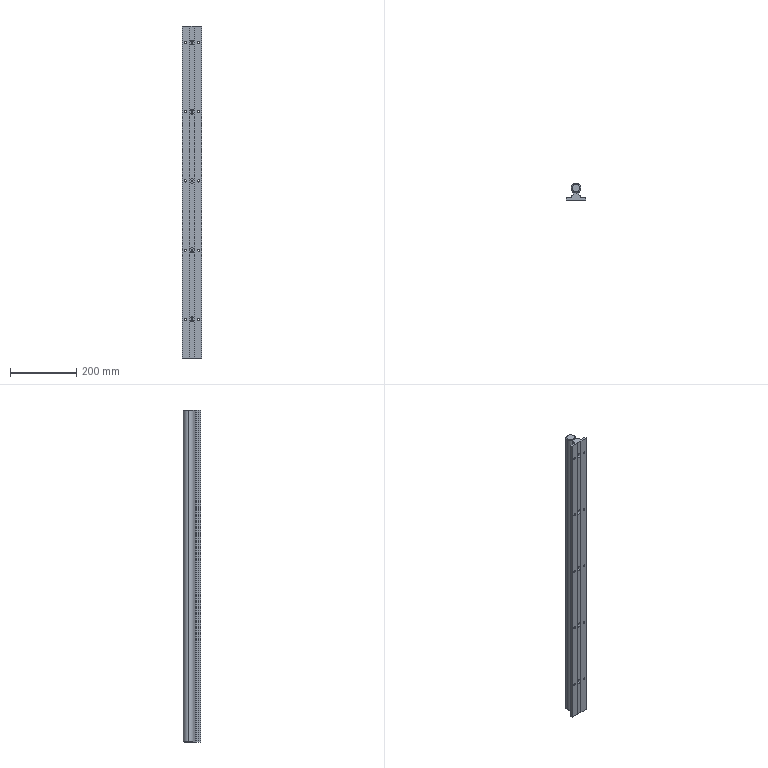Part | SolidWorks | features RevCut 2, Chamfer 1, CurvePattern 1, Extrusion 1, ICE 1, MirrorPattern 1 | 1 solid | 93 faces | box 60 x 52 x 1000 mm | volume 1438774 mm3 | cylinder 55 | plane 34 | cone 4 | commonest cylinder face diameters 6.6 x20 1.4 x10 5.6 x10 14 x10 30 x5